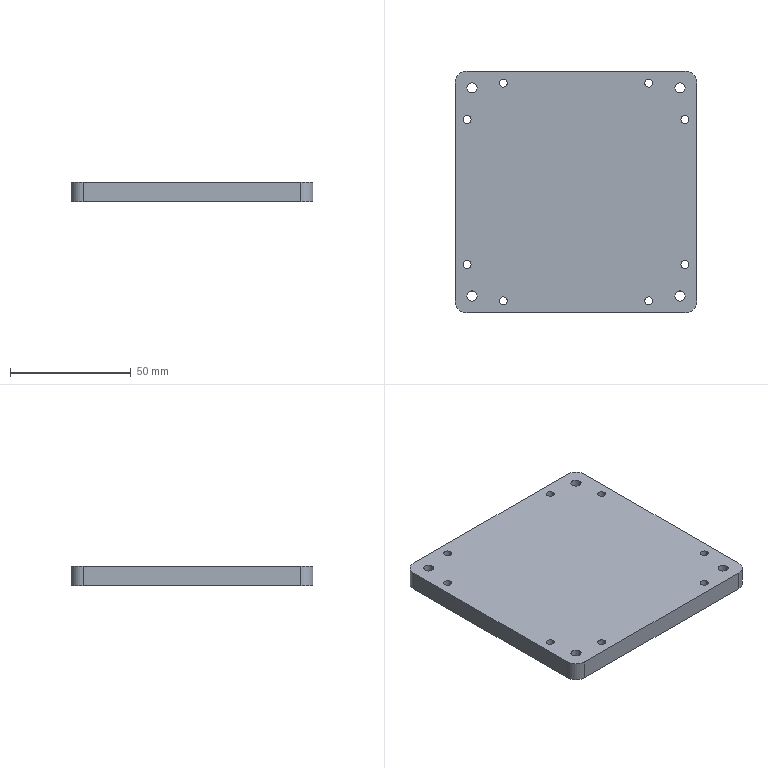Part | SolidWorks | features 3DProfileFeature 2, HoleWzd 2, Extrusion 1 | 1 solid | 34 faces | box 100 x 100 x 8 mm | volume 78838 mm3 | cylinder 28 | plane 6 | commonest cylinder face diameters 3.3 x16 4.2 x8 10 x4
STEP:
#1=CARTESIAN_POINT('',(-31.65,-45.,0.));
#2=VERTEX_POINT('',#1);
#3=CARTESIAN_POINT('',(-28.35,-45.,0.));
#4=VERTEX_POINT('',#3);
#5=CARTESIAN_POINT('',(-30.,-45.,0.));
#6=DIRECTION('',(0.,0.,1.));
#7=DIRECTION('',(1.,0.,0.));
#8=AXIS2_PLACEMENT_3D('',#5,#6,#7);
#9=CIRCLE('',#8,1.65);
#10=EDGE_CURVE('',#2,#4,#9,.T.);
#11=ORIENTED_EDGE('',*,*,#10,.F.);
#12=CARTESIAN_POINT('',(-31.65,-45.,8.));
#13=VERTEX_POINT('',#12);
#14=CARTESIAN_POINT('',(-31.65,-45.,8.));
#15=DIRECTION('',(0.,0.,1.));
#16=VECTOR('',#15,1000.);
#17=LINE('',#14,#16);
#18=EDGE_CURVE('',#2,#13,#17,.T.);
#19=ORIENTED_EDGE('',*,*,#18,.T.);
#20=CARTESIAN_POINT('',(-28.35,-45.,8.));
#21=VERTEX_POINT('',#20);
#22=CARTESIAN_POINT('',(-30.,-45.,8.));
#23=DIRECTION('',(0.,0.,1.));
#24=DIRECTION('',(1.,0.,0.));
#25=AXIS2_PLACEMENT_3D('',#22,#23,#24);
#26=CIRCLE('',#25,1.65);
#27=EDGE_CURVE('',#13,#21,#26,.T.);
#28=ORIENTED_EDGE('',*,*,#27,.T.);
#29=CARTESIAN_POINT('',(-28.35,-45.,8.));
#30=DIRECTION('',(0.,0.,1.));
#31=VECTOR('',#30,1000.);
#32=LINE('',#29,#31);
#33=EDGE_CURVE('',#4,#21,#32,.T.);
#34=ORIENTED_EDGE('',*,*,#33,.F.);
#35=EDGE_LOOP('',(#11,#19,#28,#34));
#36=FACE_OUTER_BOUND('',#35,.T.);
#37=CARTESIAN_POINT('',(-30.,-45.,8.));
#38=DIRECTION('',(0.,0.,1.));
#39=DIRECTION('',(1.,0.,0.));
#40=AXIS2_PLACEMENT_3D('',#37,#38,#39);
#41=CYLINDRICAL_SURFACE('',#40,1.65);
#42=ADVANCED_FACE('',(#36),#41,.F.);
#43=CARTESIAN_POINT('',(28.35,-45.,0.));
#44=VERTEX_POINT('',#43);
#45=CARTESIAN_POINT('',(31.65,-45.,0.));
#46=VERTEX_POINT('',#45);
#47=CARTESIAN_POINT('',(30.,-45.,0.));
#48=DIRECTION('',(0.,0.,1.));
#49=DIRECTION('',(1.,0.,0.));
#50=AXIS2_PLACEMENT_3D('',#47,#48,#49);
#51=CIRCLE('',#50,1.65);
#52=EDGE_CURVE('',#44,#46,#51,.T.);
#53=ORIENTED_EDGE('',*,*,#52,.F.);
#54=CARTESIAN_POINT('',(28.35,-45.,8.));
#55=VERTEX_POINT('',#54);
#56=CARTESIAN_POINT('',(28.35,-45.,8.));
#57=DIRECTION('',(0.,0.,1.));
#58=VECTOR('',#57,1000.);
#59=LINE('',#56,#58);
#60=EDGE_CURVE('',#44,#55,#59,.T.);
#61=ORIENTED_EDGE('',*,*,#60,.T.);
#62=CARTESIAN_POINT('',(31.65,-45.,8.));
#63=VERTEX_POINT('',#62);
#64=CARTESIAN_POINT('',(30.,-45.,8.));
#65=DIRECTION('',(0.,0.,1.));
#66=DIRECTION('',(1.,0.,0.));
#67=AXIS2_PLACEMENT_3D('',#64,#65,#66);
#68=CIRCLE('',#67,1.65);
#69=EDGE_CURVE('',#55,#63,#68,.T.);
#70=ORIENTED_EDGE('',*,*,#69,.T.);
#71=CARTESIAN_POINT('',(31.65,-45.,8.));
#72=DIRECTION('',(0.,0.,1.));
#73=VECTOR('',#72,1000.);
#74=LINE('',#71,#73);
#75=EDGE_CURVE('',#46,#63,#74,.T.);
#76=ORIENTED_EDGE('',*,*,#75,.F.);
#77=EDGE_LOOP('',(#53,#61,#70,#76));
#78=FACE_OUTER_BOUND('',#77,.T.);
#79=CARTESIAN_POINT('',(30.,-45.,8.));
#80=DIRECTION('',(0.,0.,1.));
#81=DIRECTION('',(1.,0.,0.));
#82=AXIS2_PLACEMENT_3D('',#79,#80,#81);
#83=CYLINDRICAL_SURFACE('',#82,1.65);
#84=ADVANCED_FACE('',(#78),#83,.F.);
#85=CARTESIAN_POINT('',(-46.65,-30.,0.));
#86=VERTEX_POINT('',#85);
#87=CARTESIAN_POINT('',(-43.35,-30.,0.));
#88=VERTEX_POINT('',#87);
#89=CARTESIAN_POINT('',(-45.,-30.,0.));
#90=DIRECTION('',(0.,0.,1.));
#91=DIRECTION('',(1.,0.,0.));
#92=AXIS2_PLACEMENT_3D('',#89,#90,#91);
#93=CIRCLE('',#92,1.65);
#94=EDGE_CURVE('',#86,#88,#93,.T.);
#95=ORIENTED_EDGE('',*,*,#94,.F.);
#96=CARTESIAN_POINT('',(-46.65,-30.,8.));
#97=VERTEX_POINT('',#96);
#98=CARTESIAN_POINT('',(-46.65,-30.,8.));
#99=DIRECTION('',(0.,0.,1.));
#100=VECTOR('',#99,1000.);
#101=LINE('',#98,#100);
#102=EDGE_CURVE('',#86,#97,#101,.T.);
#103=ORIENTED_EDGE('',*,*,#102,.T.);
#104=CARTESIAN_POINT('',(-43.35,-30.,8.));
#105=VERTEX_POINT('',#104);
#106=CARTESIAN_POINT('',(-45.,-30.,8.));
#107=DIRECTION('',(0.,0.,1.));
#108=DIRECTION('',(1.,0.,0.));
#109=AXIS2_PLACEMENT_3D('',#106,#107,#108);
#110=CIRCLE('',#109,1.65);
#111=EDGE_CURVE('',#97,#105,#110,.T.);
#112=ORIENTED_EDGE('',*,*,#111,.T.);
#113=CARTESIAN_POINT('',(-43.35,-30.,8.));
#114=DIRECTION('',(0.,0.,1.));
#115=VECTOR('',#114,1000.);
#116=LINE('',#113,#115);
#117=EDGE_CURVE('',#88,#105,#116,.T.);
#118=ORIENTED_EDGE('',*,*,#117,.F.);
#119=EDGE_LOOP('',(#95,#103,#112,#118));
#120=FACE_OUTER_BOUND('',#119,.T.);
#121=CARTESIAN_POINT('',(-45.,-30.,8.));
#122=DIRECTION('',(0.,0.,1.));
#123=DIRECTION('',(1.,0.,0.));
#124=AXIS2_PLACEMENT_3D('',#121,#122,#123);
#125=CYLINDRICAL_SURFACE('',#124,1.65);
#126=ADVANCED_FACE('',(#120),#125,.F.);
#127=CARTESIAN_POINT('',(-46.65,30.,0.));
#128=VERTEX_POINT('',#127);
#129=CARTESIAN_POINT('',(-43.35,30.,0.));
#130=VERTEX_POINT('',#129);
#131=CARTESIAN_POINT('',(-45.,30.,0.));
#132=DIRECTION('',(0.,0.,1.));
#133=DIRECTION('',(1.,0.,0.));
#134=AXIS2_PLACEMENT_3D('',#131,#132,#133);
#135=CIRCLE('',#134,1.65);
#136=EDGE_CURVE('',#128,#130,#135,.T.);
#137=ORIENTED_EDGE('',*,*,#136,.F.);
#138=CARTESIAN_POINT('',(-46.65,30.,8.));
#139=VERTEX_POINT('',#138);
#140=CARTESIAN_POINT('',(-46.65,30.,8.));
#141=DIRECTION('',(0.,0.,1.));
#142=VECTOR('',#141,1000.);
#143=LINE('',#140,#142);
#144=EDGE_CURVE('',#128,#139,#143,.T.);
#145=ORIENTED_EDGE('',*,*,#144,.T.);
#146=CARTESIAN_POINT('',(-43.35,30.,8.));
#147=VERTEX_POINT('',#146);
#148=CARTESIAN_POINT('',(-45.,30.,8.));
#149=DIRECTION('',(0.,0.,1.));
#150=DIRECTION('',(1.,0.,0.));
#151=AXIS2_PLACEMENT_3D('',#148,#149,#150);
#152=CIRCLE('',#151,1.65);
#153=EDGE_CURVE('',#139,#147,#152,.T.);
#154=ORIENTED_EDGE('',*,*,#153,.T.);
#155=CARTESIAN_POINT('',(-43.35,30.,8.));
#156=DIRECTION('',(0.,0.,1.));
#157=VECTOR('',#156,1000.);
#158=LINE('',#155,#157);
#159=EDGE_CURVE('',#130,#147,#158,.T.);
#160=ORIENTED_EDGE('',*,*,#159,.F.);
#161=EDGE_LOOP('',(#137,#145,#154,#160));
#162=FACE_OUTER_BOUND('',#161,.T.);
#163=CARTESIAN_POINT('',(-45.,30.,8.));
#164=DIRECTION('',(0.,0.,1.));
#165=DIRECTION('',(1.,0.,0.));
#166=AXIS2_PLACEMENT_3D('',#163,#164,#165);
#167=CYLINDRICAL_SURFACE('',#166,1.65);
#168=ADVANCED_FACE('',(#162),#167,.F.);
#169=CARTESIAN_POINT('',(43.35,30.,0.));
#170=VERTEX_POINT('',#169);
#171=CARTESIAN_POINT('',(46.65,30.,0.));
#172=VERTEX_POINT('',#171);
#173=CARTESIAN_POINT('',(45.,30.,0.));
#174=DIRECTION('',(0.,0.,1.));
#175=DIRECTION('',(1.,0.,0.));
#176=AXIS2_PLACEMENT_3D('',#173,#174,#175);
#177=CIRCLE('',#176,1.65);
#178=EDGE_CURVE('',#170,#172,#177,.T.);
#179=ORIENTED_EDGE('',*,*,#178,.F.);
#180=CARTESIAN_POINT('',(43.35,30.,8.));
#181=VERTEX_POINT('',#180);
#182=CARTESIAN_POINT('',(43.35,30.,8.));
#183=DIRECTION('',(0.,0.,1.));
#184=VECTOR('',#183,1000.);
#185=LINE('',#182,#184);
#186=EDGE_CURVE('',#170,#181,#185,.T.);
#187=ORIENTED_EDGE('',*,*,#186,.T.);
#188=CARTESIAN_POINT('',(46.65,30.,8.));
#189=VERTEX_POINT('',#188);
#190=CARTESIAN_POINT('',(45.,30.,8.));
#191=DIRECTION('',(0.,0.,1.));
#192=DIRECTION('',(1.,0.,0.));
#193=AXIS2_PLACEMENT_3D('',#190,#191,#192);
#194=CIRCLE('',#193,1.65);
#195=EDGE_CURVE('',#181,#189,#194,.T.);
#196=ORIENTED_EDGE('',*,*,#195,.T.);
#197=CARTESIAN_POINT('',(46.65,30.,8.));
#198=DIRECTION('',(0.,0.,1.));
#199=VECTOR('',#198,1000.);
#200=LINE('',#197,#199);
#201=EDGE_CURVE('',#172,#189,#200,.T.);
#202=ORIENTED_EDGE('',*,*,#201,.F.);
#203=EDGE_LOOP('',(#179,#187,#196,#202));
#204=FACE_OUTER_BOUND('',#203,.T.);
#205=CARTESIAN_POINT('',(45.,30.,8.));
#206=DIRECTION('',(0.,0.,1.));
#207=DIRECTION('',(1.,0.,0.));
#208=AXIS2_PLACEMENT_3D('',#205,#206,#207);
#209=CYLINDRICAL_SURFACE('',#208,1.65);
#210=ADVANCED_FACE('',(#204),#209,.F.);
#211=CARTESIAN_POINT('',(43.35,-30.,0.));
#212=VERTEX_POINT('',#211);
#213=CARTESIAN_POINT('',(46.65,-30.,0.));
#214=VERTEX_POINT('',#213);
#215=CARTESIAN_POINT('',(45.,-30.,0.));
#216=DIRECTION('',(0.,0.,1.));
#217=DIRECTION('',(1.,0.,0.));
#218=AXIS2_PLACEMENT_3D('',#215,#216,#217);
#219=CIRCLE('',#218,1.65);
#220=EDGE_CURVE('',#212,#214,#219,.T.);
#221=ORIENTED_EDGE('',*,*,#220,.F.);
#222=CARTESIAN_POINT('',(43.35,-30.,8.));
#223=VERTEX_POINT('',#222);
#224=CARTESIAN_POINT('',(43.35,-30.,8.));
#225=DIRECTION('',(0.,0.,1.));
#226=VECTOR('',#225,1000.);
#227=LINE('',#224,#226);
#228=EDGE_CURVE('',#212,#223,#227,.T.);
#229=ORIENTED_EDGE('',*,*,#228,.T.);
#230=CARTESIAN_POINT('',(46.65,-30.,8.));
#231=VERTEX_POINT('',#230);
#232=CARTESIAN_POINT('',(45.,-30.,8.));
#233=DIRECTION('',(0.,0.,1.));
#234=DIRECTION('',(1.,0.,0.));
#235=AXIS2_PLACEMENT_3D('',#232,#233,#234);
#236=CIRCLE('',#235,1.65);
#237=EDGE_CURVE('',#223,#231,#236,.T.);
#238=ORIENTED_EDGE('',*,*,#237,.T.);
#239=CARTESIAN_POINT('',(46.65,-30.,8.));
#240=DIRECTION('',(0.,0.,1.));
#241=VECTOR('',#240,1000.);
#242=LINE('',#239,#241);
#243=EDGE_CURVE('',#214,#231,#242,.T.);
#244=ORIENTED_EDGE('',*,*,#243,.F.);
#245=EDGE_LOOP('',(#221,#229,#238,#244));
#246=FACE_OUTER_BOUND('',#245,.T.);
#247=CARTESIAN_POINT('',(45.,-30.,8.));
#248=DIRECTION('',(0.,0.,1.));
#249=DIRECTION('',(1.,0.,0.));
#250=AXIS2_PLACEMENT_3D('',#247,#248,#249);
#251=CYLINDRICAL_SURFACE('',#250,1.65);
#252=ADVANCED_FACE('',(#246),#251,.F.);
#253=CARTESIAN_POINT('',(-31.65,45.,0.));
#254=VERTEX_POINT('',#253);
#255=CARTESIAN_POINT('',(-28.35,45.,0.));
#256=VERTEX_POINT('',#255);
#257=CARTESIAN_POINT('',(-30.,45.,0.));
#258=DIRECTION('',(0.,0.,1.));
#259=DIRECTION('',(1.,0.,0.));
#260=AXIS2_PLACEMENT_3D('',#257,#258,#259);
#261=CIRCLE('',#260,1.65);
#262=EDGE_CURVE('',#254,#256,#261,.T.);
#263=ORIENTED_EDGE('',*,*,#262,.F.);
#264=CARTESIAN_POINT('',(-31.65,45.,8.));
#265=VERTEX_POINT('',#264);
#266=CARTESIAN_POINT('',(-31.65,45.,8.));
#267=DIRECTION('',(0.,0.,1.));
#268=VECTOR('',#267,1000.);
#269=LINE('',#266,#268);
#270=EDGE_CURVE('',#254,#265,#269,.T.);
#271=ORIENTED_EDGE('',*,*,#270,.T.);
#272=CARTESIAN_POINT('',(-28.35,45.,8.));
#273=VERTEX_POINT('',#272);
#274=CARTESIAN_POINT('',(-30.,45.,8.));
#275=DIRECTION('',(0.,0.,1.));
#276=DIRECTION('',(1.,0.,0.));
#277=AXIS2_PLACEMENT_3D('',#274,#275,#276);
#278=CIRCLE('',#277,1.65);
#279=EDGE_CURVE('',#265,#273,#278,.T.);
#280=ORIENTED_EDGE('',*,*,#279,.T.);
#281=CARTESIAN_POINT('',(-28.35,45.,8.));
#282=DIRECTION('',(0.,0.,1.));
#283=VECTOR('',#282,1000.);
#284=LINE('',#281,#283);
#285=EDGE_CURVE('',#256,#273,#284,.T.);
#286=ORIENTED_EDGE('',*,*,#285,.F.);
#287=EDGE_LOOP('',(#263,#271,#280,#286));
#288=FACE_OUTER_BOUND('',#287,.T.);
#289=CARTESIAN_POINT('',(-30.,45.,8.));
#290=DIRECTION('',(0.,0.,1.));
#291=DIRECTION('',(1.,0.,0.));
#292=AXIS2_PLACEMENT_3D('',#289,#290,#291);
#293=CYLINDRICAL_SURFACE('',#292,1.65);
#294=ADVANCED_FACE('',(#288),#293,.F.);
#295=CARTESIAN_POINT('',(28.35,45.,0.));
#296=VERTEX_POINT('',#295);
#297=CARTESIAN_POINT('',(31.65,45.,0.));
#298=VERTEX_POINT('',#297);
#299=CARTESIAN_POINT('',(30.,45.,0.));
#300=DIRECTION('',(0.,0.,1.));
#301=DIRECTION('',(1.,0.,0.));
#302=AXIS2_PLACEMENT_3D('',#299,#300,#301);
#303=CIRCLE('',#302,1.65);
#304=EDGE_CURVE('',#296,#298,#303,.T.);
#305=ORIENTED_EDGE('',*,*,#304,.F.);
#306=CARTESIAN_POINT('',(28.35,45.,8.));
#307=VERTEX_POINT('',#306);
#308=CARTESIAN_POINT('',(28.35,45.,8.));
#309=DIRECTION('',(0.,0.,1.));
#310=VECTOR('',#309,1000.);
#311=LINE('',#308,#310);
#312=EDGE_CURVE('',#296,#307,#311,.T.);
#313=ORIENTED_EDGE('',*,*,#312,.T.);
#314=CARTESIAN_POINT('',(31.65,45.,8.));
#315=VERTEX_POINT('',#314);
#316=CARTESIAN_POINT('',(30.,45.,8.));
#317=DIRECTION('',(0.,0.,1.));
#318=DIRECTION('',(1.,0.,0.));
#319=AXIS2_PLACEMENT_3D('',#316,#317,#318);
#320=CIRCLE('',#319,1.65);
#321=EDGE_CURVE('',#307,#315,#320,.T.);
#322=ORIENTED_EDGE('',*,*,#321,.T.);
#323=CARTESIAN_POINT('',(31.65,45.,8.));
#324=DIRECTION('',(0.,0.,1.));
#325=VECTOR('',#324,1000.);
#326=LINE('',#323,#325);
#327=EDGE_CURVE('',#298,#315,#326,.T.);
#328=ORIENTED_EDGE('',*,*,#327,.F.);
#329=EDGE_LOOP('',(#305,#313,#322,#328));
#330=FACE_OUTER_BOUND('',#329,.T.);
#331=CARTESIAN_POINT('',(30.,45.,8.));
#332=DIRECTION('',(0.,0.,1.));
#333=DIRECTION('',(1.,0.,0.));
#334=AXIS2_PLACEMENT_3D('',#331,#332,#333);
#335=CYLINDRICAL_SURFACE('',#334,1.65);
#336=ADVANCED_FACE('',(#330),#335,.F.);
#337=CARTESIAN_POINT('',(-45.1,43.,0.));
#338=VERTEX_POINT('',#337);
#339=CARTESIAN_POINT('',(-40.9,43.,0.));
#340=VERTEX_POINT('',#339);
#341=CARTESIAN_POINT('',(-43.,43.,0.));
#342=DIRECTION('',(0.,0.,1.));
#343=DIRECTION('',(1.,0.,0.));
#344=AXIS2_PLACEMENT_3D('',#341,#342,#343);
#345=CIRCLE('',#344,2.1);
#346=EDGE_CURVE('',#338,#340,#345,.T.);
#347=ORIENTED_EDGE('',*,*,#346,.F.);
#348=CARTESIAN_POINT('',(-45.1,43.,8.));
#349=VERTEX_POINT('',#348);
#350=CARTESIAN_POINT('',(-45.1,43.,8.));
#351=DIRECTION('',(0.,0.,1.));
#352=VECTOR('',#351,1000.);
#353=LINE('',#350,#352);
#354=EDGE_CURVE('',#338,#349,#353,.T.);
#355=ORIENTED_EDGE('',*,*,#354,.T.);
#356=CARTESIAN_POINT('',(-40.9,43.,8.));
#357=VERTEX_POINT('',#356);
#358=CARTESIAN_POINT('',(-43.,43.,8.));
#359=DIRECTION('',(0.,0.,1.));
#360=DIRECTION('',(1.,0.,0.));
#361=AXIS2_PLACEMENT_3D('',#358,#359,#360);
#362=CIRCLE('',#361,2.1);
#363=EDGE_CURVE('',#349,#357,#362,.T.);
#364=ORIENTED_EDGE('',*,*,#363,.T.);
#365=CARTESIAN_POINT('',(-40.9,43.,8.));
#366=DIRECTION('',(0.,0.,1.));
#367=VECTOR('',#366,1000.);
#368=LINE('',#365,#367);
#369=EDGE_CURVE('',#340,#357,#368,.T.);
#370=ORIENTED_EDGE('',*,*,#369,.F.);
#371=EDGE_LOOP('',(#347,#355,#364,#370));
#372=FACE_OUTER_BOUND('',#371,.T.);
#373=CARTESIAN_POINT('',(-43.,43.,8.));
#374=DIRECTION('',(0.,0.,1.));
#375=DIRECTION('',(1.,0.,0.));
#376=AXIS2_PLACEMENT_3D('',#373,#374,#375);
#377=CYLINDRICAL_SURFACE('',#376,2.1);
#378=ADVANCED_FACE('',(#372),#377,.F.);
#379=CARTESIAN_POINT('',(40.9,43.,0.));
#380=VERTEX_POINT('',#379);
#381=CARTESIAN_POINT('',(45.1,43.,0.));
#382=VERTEX_POINT('',#381);
#383=CARTESIAN_POINT('',(43.,43.,0.));
#384=DIRECTION('',(0.,0.,1.));
#385=DIRECTION('',(1.,0.,0.));
#386=AXIS2_PLACEMENT_3D('',#383,#384,#385);
#387=CIRCLE('',#386,2.1);
#388=EDGE_CURVE('',#380,#382,#387,.T.);
#389=ORIENTED_EDGE('',*,*,#388,.F.);
#390=CARTESIAN_POINT('',(40.9,43.,8.));
#391=VERTEX_POINT('',#390);
#392=CARTESIAN_POINT('',(40.9,43.,8.));
#393=DIRECTION('',(0.,0.,1.));
#394=VECTOR('',#393,1000.);
#395=LINE('',#392,#394);
#396=EDGE_CURVE('',#380,#391,#395,.T.);
#397=ORIENTED_EDGE('',*,*,#396,.T.);
#398=CARTESIAN_POINT('',(45.1,43.,8.));
#399=VERTEX_POINT('',#398);
#400=CARTESIAN_POINT('',(43.,43.,8.));
#401=DIRECTION('',(0.,0.,1.));
#402=DIRECTION('',(1.,0.,0.));
#403=AXIS2_PLACEMENT_3D('',#400,#401,#402);
#404=CIRCLE('',#403,2.1);
#405=EDGE_CURVE('',#391,#399,#404,.T.);
#406=ORIENTED_EDGE('',*,*,#405,.T.);
#407=CARTESIAN_POINT('',(45.1,43.,8.));
#408=DIRECTION('',(0.,0.,1.));
#409=VECTOR('',#408,1000.);
#410=LINE('',#407,#409);
#411=EDGE_CURVE('',#382,#399,#410,.T.);
#412=ORIENTED_EDGE('',*,*,#411,.F.);
#413=EDGE_LOOP('',(#389,#397,#406,#412));
#414=FACE_OUTER_BOUND('',#413,.T.);
#415=CARTESIAN_POINT('',(43.,43.,8.));
#416=DIRECTION('',(0.,0.,1.));
#417=DIRECTION('',(1.,0.,0.));
#418=AXIS2_PLACEMENT_3D('',#415,#416,#417);
#419=CYLINDRICAL_SURFACE('',#418,2.1);
#420=ADVANCED_FACE('',(#414),#419,.F.);
#421=CARTESIAN_POINT('',(40.9,-43.,0.));
#422=VERTEX_POINT('',#421);
#423=CARTESIAN_POINT('',(45.1,-43.,0.));
#424=VERTEX_POINT('',#423);
#425=CARTESIAN_POINT('',(43.,-43.,0.));
#426=DIRECTION('',(0.,0.,1.));
#427=DIRECTION('',(1.,0.,0.));
#428=AXIS2_PLACEMENT_3D('',#425,#426,#427);
#429=CIRCLE('',#428,2.1);
#430=EDGE_CURVE('',#422,#424,#429,.T.);
#431=ORIENTED_EDGE('',*,*,#430,.F.);
#432=CARTESIAN_POINT('',(40.9,-43.,8.));
#433=VERTEX_POINT('',#432);
#434=CARTESIAN_POINT('',(40.9,-43.,8.));
#435=DIRECTION('',(0.,0.,1.));
#436=VECTOR('',#435,1000.);
#437=LINE('',#434,#436);
#438=EDGE_CURVE('',#422,#433,#437,.T.);
#439=ORIENTED_EDGE('',*,*,#438,.T.);
#440=CARTESIAN_POINT('',(45.1,-43.,8.));
#441=VERTEX_POINT('',#440);
#442=CARTESIAN_POINT('',(43.,-43.,8.));
#443=DIRECTION('',(0.,0.,1.));
#444=DIRECTION('',(1.,0.,0.));
#445=AXIS2_PLACEMENT_3D('',#442,#443,#444);
#446=CIRCLE('',#445,2.1);
#447=EDGE_CURVE('',#433,#441,#446,.T.);
#448=ORIENTED_EDGE('',*,*,#447,.T.);
#449=CARTESIAN_POINT('',(45.1,-43.,8.));
#450=DIRECTION('',(0.,0.,1.));
#451=VECTOR('',#450,1000.);
#452=LINE('',#449,#451);
#453=EDGE_CURVE('',#424,#441,#452,.T.);
#454=ORIENTED_EDGE('',*,*,#453,.F.);
#455=EDGE_LOOP('',(#431,#439,#448,#454));
#456=FACE_OUTER_BOUND('',#455,.T.);
#457=CARTESIAN_POINT('',(43.,-43.,8.));
#458=DIRECTION('',(0.,0.,1.));
#459=DIRECTION('',(1.,0.,0.));
#460=AXIS2_PLACEMENT_3D('',#457,#458,#459);
#461=CYLINDRICAL_SURFACE('',#460,2.1);
#462=ADVANCED_FACE('',(#456),#461,.F.);
#463=CARTESIAN_POINT('',(-45.1,-43.,0.));
#464=VERTEX_POINT('',#463);
#465=CARTESIAN_POINT('',(-40.9,-43.,0.));
#466=VERTEX_POINT('',#465);
#467=CARTESIAN_POINT('',(-43.,-43.,0.));
#468=DIRECTION('',(0.,0.,1.));
#469=DIRECTION('',(1.,0.,0.));
#470=AXIS2_PLACEMENT_3D('',#467,#468,#469);
#471=CIRCLE('',#470,2.1);
#472=EDGE_CURVE('',#464,#466,#471,.T.);
#473=ORIENTED_EDGE('',*,*,#472,.F.);
#474=CARTESIAN_POINT('',(-45.1,-43.,8.));
#475=VERTEX_POINT('',#474);
#476=CARTESIAN_POINT('',(-45.1,-43.,8.));
#477=DIRECTION('',(0.,0.,1.));
#478=VECTOR('',#477,1000.);
#479=LINE('',#476,#478);
#480=EDGE_CURVE('',#464,#475,#479,.T.);
#481=ORIENTED_EDGE('',*,*,#480,.T.);
#482=CARTESIAN_POINT('',(-40.9,-43.,8.));
#483=VERTEX_POINT('',#482);
#484=CARTESIAN_POINT('',(-43.,-43.,8.));
#485=DIRECTION('',(0.,0.,1.));
#486=DIRECTION('',(1.,0.,0.));
#487=AXIS2_PLACEMENT_3D('',#484,#485,#486);
#488=CIRCLE('',#487,2.1);
#489=EDGE_CURVE('',#475,#483,#488,.T.);
#490=ORIENTED_EDGE('',*,*,#489,.T.);
#491=CARTESIAN_POINT('',(-40.9,-43.,8.));
#492=DIRECTION('',(0.,0.,1.));
#493=VECTOR('',#492,1000.);
#494=LINE('',#491,#493);
#495=EDGE_CURVE('',#466,#483,#494,.T.);
#496=ORIENTED_EDGE('',*,*,#495,.F.);
#497=EDGE_LOOP('',(#473,#481,#490,#496));
#498=FACE_OUTER_BOUND('',#497,.T.);
#499=CARTESIAN_POINT('',(-43.,-43.,8.));
#500=DIRECTION('',(0.,0.,1.));
#501=DIRECTION('',(1.,0.,0.));
#502=AXIS2_PLACEMENT_3D('',#499,#500,#501);
#503=CYLINDRICAL_SURFACE('',#502,2.1);
#504=ADVANCED_FACE('',(#498),#503,.F.);
#505=CARTESIAN_POINT('',(45.,-50.,0.));
#506=VERTEX_POINT('',#505);
#507=CARTESIAN_POINT('',(50.,-45.,0.));
#508=VERTEX_POINT('',#507);
#509=CARTESIAN_POINT('',(45.,-45.,0.));
#510=DIRECTION('',(0.,0.,1.));
#511=DIRECTION('',(1.,0.,0.));
#512=AXIS2_PLACEMENT_3D('',#509,#510,#511);
#513=CIRCLE('',#512,5.);
#514=EDGE_CURVE('',#506,#508,#513,.T.);
#515=ORIENTED_EDGE('',*,*,#514,.T.);
#516=CARTESIAN_POINT('',(50.,-45.,8.));
#517=VERTEX_POINT('',#516);
#518=CARTESIAN_POINT('',(50.,-45.,8.));
#519=DIRECTION('',(0.,0.,-1.));
#520=VECTOR('',#519,1000.);
#521=LINE('',#518,#520);
#522=EDGE_CURVE('',#517,#508,#521,.T.);
#523=ORIENTED_EDGE('',*,*,#522,.F.);
#524=CARTESIAN_POINT('',(45.,-50.,8.));
#525=VERTEX_POINT('',#524);
#526=CARTESIAN_POINT('',(45.,-45.,8.));
#527=DIRECTION('',(0.,0.,1.));
#528=DIRECTION('',(1.,0.,0.));
#529=AXIS2_PLACEMENT_3D('',#526,#527,#528);
#530=CIRCLE('',#529,5.);
#531=EDGE_CURVE('',#525,#517,#530,.T.);
#532=ORIENTED_EDGE('',*,*,#531,.F.);
#533=CARTESIAN_POINT('',(45.,-50.,8.));
#534=DIRECTION('',(0.,0.,-1.));
#535=VECTOR('',#534,1000.);
#536=LINE('',#533,#535);
#537=EDGE_CURVE('',#525,#506,#536,.T.);
#538=ORIENTED_EDGE('',*,*,#537,.T.);
#539=EDGE_LOOP('',(#515,#523,#532,#538));
#540=FACE_OUTER_BOUND('',#539,.T.);
#541=CARTESIAN_POINT('',(45.,-45.,8.));
#542=DIRECTION('',(0.,0.,-1.));
#543=DIRECTION('',(-1.,0.,0.));
#544=AXIS2_PLACEMENT_3D('',#541,#542,#543);
#545=CYLINDRICAL_SURFACE('',#544,5.);
#546=ADVANCED_FACE('',(#540),#545,.T.);
#547=CARTESIAN_POINT('',(50.,45.,0.));
#548=VERTEX_POINT('',#547);
#549=CARTESIAN_POINT('',(50.,45.,0.));
#550=DIRECTION('',(0.,1.,0.));
#551=VECTOR('',#550,1000.);
#552=LINE('',#549,#551);
#553=EDGE_CURVE('',#508,#548,#552,.T.);
#554=ORIENTED_EDGE('',*,*,#553,.T.);
#555=CARTESIAN_POINT('',(50.,45.,8.));
#556=VERTEX_POINT('',#555);
#557=CARTESIAN_POINT('',(50.,45.,8.));
#558=DIRECTION('',(0.,0.,-1.));
#559=VECTOR('',#558,1000.);
#560=LINE('',#557,#559);
#561=EDGE_CURVE('',#556,#548,#560,.T.);
#562=ORIENTED_EDGE('',*,*,#561,.F.);
#563=CARTESIAN_POINT('',(50.,45.,8.));
#564=DIRECTION('',(0.,1.,0.));
#565=VECTOR('',#564,1000.);
#566=LINE('',#563,#565);
#567=EDGE_CURVE('',#517,#556,#566,.T.);
#568=ORIENTED_EDGE('',*,*,#567,.F.);
#569=ORIENTED_EDGE('',*,*,#522,.T.);
#570=EDGE_LOOP('',(#554,#562,#568,#569));
#571=FACE_OUTER_BOUND('',#570,.T.);
#572=CARTESIAN_POINT('',(50.,45.,8.));
#573=DIRECTION('',(-1.,0.,0.));
#574=DIRECTION('',(0.,-1.,0.));
#575=AXIS2_PLACEMENT_3D('',#572,#573,#574);
#576=PLANE('',#575);
#577=ADVANCED_FACE('',(#571),#576,.F.);
#578=CARTESIAN_POINT('',(45.,50.,0.));
#579=VERTEX_POINT('',#578);
#580=CARTESIAN_POINT('',(45.,45.,0.));
#581=DIRECTION('',(0.,0.,1.));
#582=DIRECTION('',(-1.,0.,0.));
#583=AXIS2_PLACEMENT_3D('',#580,#581,#582);
#584=CIRCLE('',#583,5.);
#585=EDGE_CURVE('',#548,#579,#584,.T.);
#586=ORIENTED_EDGE('',*,*,#585,.T.);
#587=CARTESIAN_POINT('',(45.,50.,8.));
#588=VERTEX_POINT('',#587);
#589=CARTESIAN_POINT('',(45.,50.,8.));
#590=DIRECTION('',(0.,0.,-1.));
#591=VECTOR('',#590,1000.);
#592=LINE('',#589,#591);
#593=EDGE_CURVE('',#588,#579,#592,.T.);
#594=ORIENTED_EDGE('',*,*,#593,.F.);
#595=CARTESIAN_POINT('',(45.,45.,8.));
#596=DIRECTION('',(0.,0.,1.));
#597=DIRECTION('',(-1.,0.,0.));
#598=AXIS2_PLACEMENT_3D('',#595,#596,#597);
#599=CIRCLE('',#598,5.);
#600=EDGE_CURVE('',#556,#588,#599,.T.);
#601=ORIENTED_EDGE('',*,*,#600,.F.);
#602=ORIENTED_EDGE('',*,*,#561,.T.);
#603=EDGE_LOOP('',(#586,#594,#601,#602));
#604=FACE_OUTER_BOUND('',#603,.T.);
#605=CARTESIAN_POINT('',(45.,45.,8.));
#606=DIRECTION('',(0.,0.,-1.));
#607=DIRECTION('',(-1.,0.,0.));
#608=AXIS2_PLACEMENT_3D('',#605,#606,#607);
#609=CYLINDRICAL_SURFACE('',#608,5.);
#610=ADVANCED_FACE('',(#604),#609,.T.);
#611=CARTESIAN_POINT('',(-45.,50.,0.));
#612=VERTEX_POINT('',#611);
#613=CARTESIAN_POINT('',(-45.,50.,0.));
#614=DIRECTION('',(-1.,0.,0.));
#615=VECTOR('',#614,1000.);
#616=LINE('',#613,#615);
#617=EDGE_CURVE('',#579,#612,#616,.T.);
#618=ORIENTED_EDGE('',*,*,#617,.T.);
#619=CARTESIAN_POINT('',(-45.,50.,8.));
#620=VERTEX_POINT('',#619);
#621=CARTESIAN_POINT('',(-45.,50.,8.));
#622=DIRECTION('',(0.,0.,-1.));
#623=VECTOR('',#622,1000.);
#624=LINE('',#621,#623);
#625=EDGE_CURVE('',#620,#612,#624,.T.);
#626=ORIENTED_EDGE('',*,*,#625,.F.);
#627=CARTESIAN_POINT('',(-45.,50.,8.));
#628=DIRECTION('',(-1.,0.,0.));
#629=VECTOR('',#628,1000.);
#630=LINE('',#627,#629);
#631=EDGE_CURVE('',#588,#620,#630,.T.);
#632=ORIENTED_EDGE('',*,*,#631,.F.);
#633=ORIENTED_EDGE('',*,*,#593,.T.);
#634=EDGE_LOOP('',(#618,#626,#632,#633));
#635=FACE_OUTER_BOUND('',#634,.T.);
#636=CARTESIAN_POINT('',(-45.,50.,8.));
#637=DIRECTION('',(0.,-1.,0.));
#638=DIRECTION('',(0.,0.,-1.));
#639=AXIS2_PLACEMENT_3D('',#636,#637,#638);
#640=PLANE('',#639);
#641=ADVANCED_FACE('',(#635),#640,.F.);
#642=CARTESIAN_POINT('',(-50.,45.,0.));
#643=VERTEX_POINT('',#642);
#644=CARTESIAN_POINT('',(-45.,45.,0.));
#645=DIRECTION('',(0.,0.,1.));
#646=DIRECTION('',(1.,0.,0.));
#647=AXIS2_PLACEMENT_3D('',#644,#645,#646);
#648=CIRCLE('',#647,5.);
#649=EDGE_CURVE('',#612,#643,#648,.T.);
#650=ORIENTED_EDGE('',*,*,#649,.T.);
#651=CARTESIAN_POINT('',(-50.,45.,8.));
#652=VERTEX_POINT('',#651);
#653=CARTESIAN_POINT('',(-50.,45.,8.));
#654=DIRECTION('',(0.,0.,-1.));
#655=VECTOR('',#654,1000.);
#656=LINE('',#653,#655);
#657=EDGE_CURVE('',#652,#643,#656,.T.);
#658=ORIENTED_EDGE('',*,*,#657,.F.);
#659=CARTESIAN_POINT('',(-45.,45.,8.));
#660=DIRECTION('',(0.,0.,1.));
#661=DIRECTION('',(1.,0.,0.));
#662=AXIS2_PLACEMENT_3D('',#659,#660,#661);
#663=CIRCLE('',#662,5.);
#664=EDGE_CURVE('',#620,#652,#663,.T.);
#665=ORIENTED_EDGE('',*,*,#664,.F.);
#666=ORIENTED_EDGE('',*,*,#625,.T.);
#667=EDGE_LOOP('',(#650,#658,#665,#666));
#668=FACE_OUTER_BOUND('',#667,.T.);
#669=CARTESIAN_POINT('',(-45.,45.,8.));
#670=DIRECTION('',(0.,0.,-1.));
#671=DIRECTION('',(-1.,0.,0.));
#672=AXIS2_PLACEMENT_3D('',#669,#670,#671);
#673=CYLINDRICAL_SURFACE('',#672,5.);
#674=ADVANCED_FACE('',(#668),#673,.T.);
#675=CARTESIAN_POINT('',(-50.,-45.,0.));
#676=VERTEX_POINT('',#675);
#677=CARTESIAN_POINT('',(-50.,45.,0.));
#678=DIRECTION('',(0.,-1.,0.));
#679=VECTOR('',#678,1000.);
#680=LINE('',#677,#679);
#681=EDGE_CURVE('',#643,#676,#680,.T.);
#682=ORIENTED_EDGE('',*,*,#681,.T.);
#683=CARTESIAN_POINT('',(-50.,-45.,8.));
#684=VERTEX_POINT('',#683);
#685=CARTESIAN_POINT('',(-50.,-45.,8.));
#686=DIRECTION('',(0.,0.,-1.));
#687=VECTOR('',#686,1000.);
#688=LINE('',#685,#687);
#689=EDGE_CURVE('',#684,#676,#688,.T.);
#690=ORIENTED_EDGE('',*,*,#689,.F.);
#691=CARTESIAN_POINT('',(-50.,45.,8.));
#692=DIRECTION('',(0.,-1.,0.));
#693=VECTOR('',#692,1000.);
#694=LINE('',#691,#693);
#695=EDGE_CURVE('',#652,#684,#694,.T.);
#696=ORIENTED_EDGE('',*,*,#695,.F.);
#697=ORIENTED_EDGE('',*,*,#657,.T.);
#698=EDGE_LOOP('',(#682,#690,#696,#697));
#699=FACE_OUTER_BOUND('',#698,.T.);
#700=CARTESIAN_POINT('',(-50.,45.,8.));
#701=DIRECTION('',(1.,0.,0.));
#702=DIRECTION('',(0.,1.,0.));
#703=AXIS2_PLACEMENT_3D('',#700,#701,#702);
#704=PLANE('',#703);
#705=ADVANCED_FACE('',(#699),#704,.F.);
#706=CARTESIAN_POINT('',(-45.,-50.,0.));
#707=VERTEX_POINT('',#706);
#708=CARTESIAN_POINT('',(-45.,-45.,0.));
#709=DIRECTION('',(0.,0.,1.));
#710=DIRECTION('',(1.,0.,0.));
#711=AXIS2_PLACEMENT_3D('',#708,#709,#710);
#712=CIRCLE('',#711,5.);
#713=EDGE_CURVE('',#676,#707,#712,.T.);
#714=ORIENTED_EDGE('',*,*,#713,.T.);
#715=CARTESIAN_POINT('',(-45.,-50.,8.));
#716=VERTEX_POINT('',#715);
#717=CARTESIAN_POINT('',(-45.,-50.,8.));
#718=DIRECTION('',(0.,0.,-1.));
#719=VECTOR('',#718,1000.);
#720=LINE('',#717,#719);
#721=EDGE_CURVE('',#716,#707,#720,.T.);
#722=ORIENTED_EDGE('',*,*,#721,.F.);
#723=CARTESIAN_POINT('',(-45.,-45.,8.));
#724=DIRECTION('',(0.,0.,1.));
#725=DIRECTION('',(1.,0.,0.));
#726=AXIS2_PLACEMENT_3D('',#723,#724,#725);
#727=CIRCLE('',#726,5.);
#728=EDGE_CURVE('',#684,#716,#727,.T.);
#729=ORIENTED_EDGE('',*,*,#728,.F.);
#730=ORIENTED_EDGE('',*,*,#689,.T.);
#731=EDGE_LOOP('',(#714,#722,#729,#730));
#732=FACE_OUTER_BOUND('',#731,.T.);
#733=CARTESIAN_POINT('',(-45.,-45.,8.));
#734=DIRECTION('',(0.,0.,-1.));
#735=DIRECTION('',(-1.,0.,0.));
#736=AXIS2_PLACEMENT_3D('',#733,#734,#735);
#737=CYLINDRICAL_SURFACE('',#736,5.);
#738=ADVANCED_FACE('',(#732),#737,.T.);
#739=CARTESIAN_POINT('',(-45.,-50.,0.));
#740=DIRECTION('',(1.,0.,0.));
#741=VECTOR('',#740,1000.);
#742=LINE('',#739,#741);
#743=EDGE_CURVE('',#707,#506,#742,.T.);
#744=ORIENTED_EDGE('',*,*,#743,.T.);
#745=ORIENTED_EDGE('',*,*,#537,.F.);
#746=CARTESIAN_POINT('',(-45.,-50.,8.));
#747=DIRECTION('',(1.,0.,0.));
#748=VECTOR('',#747,1000.);
#749=LINE('',#746,#748);
#750=EDGE_CURVE('',#716,#525,#749,.T.);
#751=ORIENTED_EDGE('',*,*,#750,.F.);
#752=ORIENTED_EDGE('',*,*,#721,.T.);
#753=EDGE_LOOP('',(#744,#745,#751,#752));
#754=FACE_OUTER_BOUND('',#753,.T.);
#755=CARTESIAN_POINT('',(-45.,-50.,8.));
#756=DIRECTION('',(0.,1.,0.));
#757=DIRECTION('',(0.,0.,1.));
#758=AXIS2_PLACEMENT_3D('',#755,#756,#757);
#759=PLANE('',#758);
#760=ADVANCED_FACE('',(#754),#759,.F.);
#761=CARTESIAN_POINT('',(-30.,-45.,8.));
#762=DIRECTION('',(0.,0.,1.));
#763=DIRECTION('',(1.,0.,0.));
#764=AXIS2_PLACEMENT_3D('',#761,#762,#763);
#765=CIRCLE('',#764,1.65);
#766=EDGE_CURVE('',#21,#13,#765,.T.);
#767=ORIENTED_EDGE('',*,*,#766,.F.);
#768=ORIENTED_EDGE('',*,*,#27,.F.);
#769=EDGE_LOOP('',(#767,#768));
#770=FACE_BOUND('',#769,.T.);
#771=CARTESIAN_POINT('',(30.,-45.,8.));
#772=DIRECTION('',(0.,0.,1.));
#773=DIRECTION('',(1.,0.,0.));
#774=AXIS2_PLACEMENT_3D('',#771,#772,#773);
#775=CIRCLE('',#774,1.65);
#776=EDGE_CURVE('',#63,#55,#775,.T.);
#777=ORIENTED_EDGE('',*,*,#776,.F.);
#778=ORIENTED_EDGE('',*,*,#69,.F.);
#779=EDGE_LOOP('',(#777,#778));
#780=FACE_BOUND('',#779,.T.);
#781=CARTESIAN_POINT('',(-45.,-30.,8.));
#782=DIRECTION('',(0.,0.,1.));
#783=DIRECTION('',(1.,0.,0.));
#784=AXIS2_PLACEMENT_3D('',#781,#782,#783);
#785=CIRCLE('',#784,1.65);
#786=EDGE_CURVE('',#105,#97,#785,.T.);
#787=ORIENTED_EDGE('',*,*,#786,.F.);
#788=ORIENTED_EDGE('',*,*,#111,.F.);
#789=EDGE_LOOP('',(#787,#788));
#790=FACE_BOUND('',#789,.T.);
#791=CARTESIAN_POINT('',(-45.,30.,8.));
#792=DIRECTION('',(0.,0.,1.));
#793=DIRECTION('',(1.,0.,0.));
#794=AXIS2_PLACEMENT_3D('',#791,#792,#793);
#795=CIRCLE('',#794,1.65);
#796=EDGE_CURVE('',#147,#139,#795,.T.);
#797=ORIENTED_EDGE('',*,*,#796,.F.);
#798=ORIENTED_EDGE('',*,*,#153,.F.);
#799=EDGE_LOOP('',(#797,#798));
#800=FACE_BOUND('',#799,.T.);
#801=CARTESIAN_POINT('',(45.,30.,8.));
#802=DIRECTION('',(0.,0.,1.));
#803=DIRECTION('',(1.,0.,0.));
#804=AXIS2_PLACEMENT_3D('',#801,#802,#803);
#805=CIRCLE('',#804,1.65);
#806=EDGE_CURVE('',#189,#181,#805,.T.);
#807=ORIENTED_EDGE('',*,*,#806,.F.);
#808=ORIENTED_EDGE('',*,*,#195,.F.);
#809=EDGE_LOOP('',(#807,#808));
#810=FACE_BOUND('',#809,.T.);
#811=CARTESIAN_POINT('',(45.,-30.,8.));
#812=DIRECTION('',(0.,0.,1.));
#813=DIRECTION('',(1.,0.,0.));
#814=AXIS2_PLACEMENT_3D('',#811,#812,#813);
#815=CIRCLE('',#814,1.65);
#816=EDGE_CURVE('',#231,#223,#815,.T.);
#817=ORIENTED_EDGE('',*,*,#816,.F.);
#818=ORIENTED_EDGE('',*,*,#237,.F.);
#819=EDGE_LOOP('',(#817,#818));
#820=FACE_BOUND('',#819,.T.);
#821=CARTESIAN_POINT('',(-30.,45.,8.));
#822=DIRECTION('',(0.,0.,1.));
#823=DIRECTION('',(1.,0.,0.));
#824=AXIS2_PLACEMENT_3D('',#821,#822,#823);
#825=CIRCLE('',#824,1.65);
#826=EDGE_CURVE('',#273,#265,#825,.T.);
#827=ORIENTED_EDGE('',*,*,#826,.F.);
#828=ORIENTED_EDGE('',*,*,#279,.F.);
#829=EDGE_LOOP('',(#827,#828));
#830=FACE_BOUND('',#829,.T.);
#831=CARTESIAN_POINT('',(30.,45.,8.));
#832=DIRECTION('',(0.,0.,1.));
#833=DIRECTION('',(1.,0.,0.));
#834=AXIS2_PLACEMENT_3D('',#831,#832,#833);
#835=CIRCLE('',#834,1.65);
#836=EDGE_CURVE('',#315,#307,#835,.T.);
#837=ORIENTED_EDGE('',*,*,#836,.F.);
#838=ORIENTED_EDGE('',*,*,#321,.F.);
#839=EDGE_LOOP('',(#837,#838));
#840=FACE_BOUND('',#839,.T.);
#841=CARTESIAN_POINT('',(-43.,43.,8.));
#842=DIRECTION('',(0.,0.,1.));
#843=DIRECTION('',(1.,0.,0.));
#844=AXIS2_PLACEMENT_3D('',#841,#842,#843);
#845=CIRCLE('',#844,2.1);
#846=EDGE_CURVE('',#357,#349,#845,.T.);
#847=ORIENTED_EDGE('',*,*,#846,.F.);
#848=ORIENTED_EDGE('',*,*,#363,.F.);
#849=EDGE_LOOP('',(#847,#848));
#850=FACE_BOUND('',#849,.T.);
#851=CARTESIAN_POINT('',(43.,43.,8.));
#852=DIRECTION('',(0.,0.,1.));
#853=DIRECTION('',(1.,0.,0.));
#854=AXIS2_PLACEMENT_3D('',#851,#852,#853);
#855=CIRCLE('',#854,2.1);
#856=EDGE_CURVE('',#399,#391,#855,.T.);
#857=ORIENTED_EDGE('',*,*,#856,.F.);
#858=ORIENTED_EDGE('',*,*,#405,.F.);
#859=EDGE_LOOP('',(#857,#858));
#860=FACE_BOUND('',#859,.T.);
#861=CARTESIAN_POINT('',(43.,-43.,8.));
#862=DIRECTION('',(0.,0.,1.));
#863=DIRECTION('',(1.,0.,0.));
#864=AXIS2_PLACEMENT_3D('',#861,#862,#863);
#865=CIRCLE('',#864,2.1);
#866=EDGE_CURVE('',#441,#433,#865,.T.);
#867=ORIENTED_EDGE('',*,*,#866,.F.);
#868=ORIENTED_EDGE('',*,*,#447,.F.);
#869=EDGE_LOOP('',(#867,#868));
#870=FACE_BOUND('',#869,.T.);
#871=CARTESIAN_POINT('',(-43.,-43.,8.));
#872=DIRECTION('',(0.,0.,1.));
#873=DIRECTION('',(1.,0.,0.));
#874=AXIS2_PLACEMENT_3D('',#871,#872,#873);
#875=CIRCLE('',#874,2.1);
#876=EDGE_CURVE('',#483,#475,#875,.T.);
#877=ORIENTED_EDGE('',*,*,#876,.F.);
#878=ORIENTED_EDGE('',*,*,#489,.F.);
#879=EDGE_LOOP('',(#877,#878));
#880=FACE_BOUND('',#879,.T.);
#881=ORIENTED_EDGE('',*,*,#531,.T.);
#882=ORIENTED_EDGE('',*,*,#567,.T.);
#883=ORIENTED_EDGE('',*,*,#600,.T.);
#884=ORIENTED_EDGE('',*,*,#631,.T.);
#885=ORIENTED_EDGE('',*,*,#664,.T.);
#886=ORIENTED_EDGE('',*,*,#695,.T.);
#887=ORIENTED_EDGE('',*,*,#728,.T.);
#888=ORIENTED_EDGE('',*,*,#750,.T.);
#889=EDGE_LOOP('',(#881,#882,#883,#884,#885,#886,#887,#888));
#890=FACE_OUTER_BOUND('',#889,.T.);
#891=CARTESIAN_POINT('',(45.,-45.,8.));
#892=DIRECTION('',(0.,0.,1.));
#893=DIRECTION('',(1.,0.,0.));
#894=AXIS2_PLACEMENT_3D('',#891,#892,#893);
#895=PLANE('',#894);
#896=ADVANCED_FACE('',(#770,#780,#790,#800,#810,#820,#830,#840,#850,#860,#870,#880,#890),#895,.T.);
#897=CARTESIAN_POINT('',(-30.,-45.,0.));
#898=DIRECTION('',(0.,0.,1.));
#899=DIRECTION('',(1.,0.,0.));
#900=AXIS2_PLACEMENT_3D('',#897,#898,#899);
#901=CIRCLE('',#900,1.65);
#902=EDGE_CURVE('',#4,#2,#901,.T.);
#903=ORIENTED_EDGE('',*,*,#902,.T.);
#904=ORIENTED_EDGE('',*,*,#10,.T.);
#905=EDGE_LOOP('',(#903,#904));
#906=FACE_BOUND('',#905,.T.);
#907=CARTESIAN_POINT('',(30.,-45.,0.));
#908=DIRECTION('',(0.,0.,1.));
#909=DIRECTION('',(1.,0.,0.));
#910=AXIS2_PLACEMENT_3D('',#907,#908,#909);
#911=CIRCLE('',#910,1.65);
#912=EDGE_CURVE('',#46,#44,#911,.T.);
#913=ORIENTED_EDGE('',*,*,#912,.T.);
#914=ORIENTED_EDGE('',*,*,#52,.T.);
#915=EDGE_LOOP('',(#913,#914));
#916=FACE_BOUND('',#915,.T.);
#917=CARTESIAN_POINT('',(-45.,-30.,0.));
#918=DIRECTION('',(0.,0.,1.));
#919=DIRECTION('',(1.,0.,0.));
#920=AXIS2_PLACEMENT_3D('',#917,#918,#919);
#921=CIRCLE('',#920,1.65);
#922=EDGE_CURVE('',#88,#86,#921,.T.);
#923=ORIENTED_EDGE('',*,*,#922,.T.);
#924=ORIENTED_EDGE('',*,*,#94,.T.);
#925=EDGE_LOOP('',(#923,#924));
#926=FACE_BOUND('',#925,.T.);
#927=CARTESIAN_POINT('',(-45.,30.,0.));
#928=DIRECTION('',(0.,0.,1.));
#929=DIRECTION('',(1.,0.,0.));
#930=AXIS2_PLACEMENT_3D('',#927,#928,#929);
#931=CIRCLE('',#930,1.65);
#932=EDGE_CURVE('',#130,#128,#931,.T.);
#933=ORIENTED_EDGE('',*,*,#932,.T.);
#934=ORIENTED_EDGE('',*,*,#136,.T.);
#935=EDGE_LOOP('',(#933,#934));
#936=FACE_BOUND('',#935,.T.);
#937=CARTESIAN_POINT('',(45.,30.,0.));
#938=DIRECTION('',(0.,0.,1.));
#939=DIRECTION('',(1.,0.,0.));
#940=AXIS2_PLACEMENT_3D('',#937,#938,#939);
#941=CIRCLE('',#940,1.65);
#942=EDGE_CURVE('',#172,#170,#941,.T.);
#943=ORIENTED_EDGE('',*,*,#942,.T.);
#944=ORIENTED_EDGE('',*,*,#178,.T.);
#945=EDGE_LOOP('',(#943,#944));
#946=FACE_BOUND('',#945,.T.);
#947=CARTESIAN_POINT('',(45.,-30.,0.));
#948=DIRECTION('',(0.,0.,1.));
#949=DIRECTION('',(1.,0.,0.));
#950=AXIS2_PLACEMENT_3D('',#947,#948,#949);
#951=CIRCLE('',#950,1.65);
#952=EDGE_CURVE('',#214,#212,#951,.T.);
#953=ORIENTED_EDGE('',*,*,#952,.T.);
#954=ORIENTED_EDGE('',*,*,#220,.T.);
#955=EDGE_LOOP('',(#953,#954));
#956=FACE_BOUND('',#955,.T.);
#957=CARTESIAN_POINT('',(-30.,45.,0.));
#958=DIRECTION('',(0.,0.,1.));
#959=DIRECTION('',(1.,0.,0.));
#960=AXIS2_PLACEMENT_3D('',#957,#958,#959);
#961=CIRCLE('',#960,1.65);
#962=EDGE_CURVE('',#256,#254,#961,.T.);
#963=ORIENTED_EDGE('',*,*,#962,.T.);
#964=ORIENTED_EDGE('',*,*,#262,.T.);
#965=EDGE_LOOP('',(#963,#964));
#966=FACE_BOUND('',#965,.T.);
#967=CARTESIAN_POINT('',(30.,45.,0.));
#968=DIRECTION('',(0.,0.,1.));
#969=DIRECTION('',(1.,0.,0.));
#970=AXIS2_PLACEMENT_3D('',#967,#968,#969);
#971=CIRCLE('',#970,1.65);
#972=EDGE_CURVE('',#298,#296,#971,.T.);
#973=ORIENTED_EDGE('',*,*,#972,.T.);
#974=ORIENTED_EDGE('',*,*,#304,.T.);
#975=EDGE_LOOP('',(#973,#974));
#976=FACE_BOUND('',#975,.T.);
#977=CARTESIAN_POINT('',(-43.,43.,0.));
#978=DIRECTION('',(0.,0.,1.));
#979=DIRECTION('',(1.,0.,0.));
#980=AXIS2_PLACEMENT_3D('',#977,#978,#979);
#981=CIRCLE('',#980,2.1);
#982=EDGE_CURVE('',#340,#338,#981,.T.);
#983=ORIENTED_EDGE('',*,*,#982,.T.);
#984=ORIENTED_EDGE('',*,*,#346,.T.);
#985=EDGE_LOOP('',(#983,#984));
#986=FACE_BOUND('',#985,.T.);
#987=CARTESIAN_POINT('',(43.,43.,0.));
#988=DIRECTION('',(0.,0.,1.));
#989=DIRECTION('',(1.,0.,0.));
#990=AXIS2_PLACEMENT_3D('',#987,#988,#989);
#991=CIRCLE('',#990,2.1);
#992=EDGE_CURVE('',#382,#380,#991,.T.);
#993=ORIENTED_EDGE('',*,*,#992,.T.);
#994=ORIENTED_EDGE('',*,*,#388,.T.);
#995=EDGE_LOOP('',(#993,#994));
#996=FACE_BOUND('',#995,.T.);
#997=CARTESIAN_POINT('',(43.,-43.,0.));
#998=DIRECTION('',(0.,0.,1.));
#999=DIRECTION('',(1.,0.,0.));
#1000=AXIS2_PLACEMENT_3D('',#997,#998,#999);
#1001=CIRCLE('',#1000,2.1);
#1002=EDGE_CURVE('',#424,#422,#1001,.T.);
#1003=ORIENTED_EDGE('',*,*,#1002,.T.);
#1004=ORIENTED_EDGE('',*,*,#430,.T.);
#1005=EDGE_LOOP('',(#1003,#1004));
#1006=FACE_BOUND('',#1005,.T.);
#1007=CARTESIAN_POINT('',(-43.,-43.,0.));
#1008=DIRECTION('',(0.,0.,1.));
#1009=DIRECTION('',(1.,0.,0.));
#1010=AXIS2_PLACEMENT_3D('',#1007,#1008,#1009);
#1011=CIRCLE('',#1010,2.1);
#1012=EDGE_CURVE('',#466,#464,#1011,.T.);
#1013=ORIENTED_EDGE('',*,*,#1012,.T.);
#1014=ORIENTED_EDGE('',*,*,#472,.T.);
#1015=EDGE_LOOP('',(#1013,#1014));
#1016=FACE_BOUND('',#1015,.T.);
#1017=ORIENTED_EDGE('',*,*,#514,.F.);
#1018=ORIENTED_EDGE('',*,*,#743,.F.);
#1019=ORIENTED_EDGE('',*,*,#713,.F.);
#1020=ORIENTED_EDGE('',*,*,#681,.F.);
#1021=ORIENTED_EDGE('',*,*,#649,.F.);
#1022=ORIENTED_EDGE('',*,*,#617,.F.);
#1023=ORIENTED_EDGE('',*,*,#585,.F.);
#1024=ORIENTED_EDGE('',*,*,#553,.F.);
#1025=EDGE_LOOP('',(#1017,#1018,#1019,#1020,#1021,#1022,#1023,#1024));
#1026=FACE_OUTER_BOUND('',#1025,.T.);
#1027=CARTESIAN_POINT('',(45.,-45.,0.));
#1028=DIRECTION('',(0.,0.,1.));
#1029=DIRECTION('',(1.,0.,0.));
#1030=AXIS2_PLACEMENT_3D('',#1027,#1028,#1029);
#1031=PLANE('',#1030);
#1032=ADVANCED_FACE('',(#906,#916,#926,#936,#946,#956,#966,#976,#986,#996,#1006,#1016,#1026),#1031,.F.);
#1033=ORIENTED_EDGE('',*,*,#480,.F.);
#1034=ORIENTED_EDGE('',*,*,#1012,.F.);
#1035=ORIENTED_EDGE('',*,*,#495,.T.);
#1036=ORIENTED_EDGE('',*,*,#876,.T.);
#1037=EDGE_LOOP('',(#1033,#1034,#1035,#1036));
#1038=FACE_OUTER_BOUND('',#1037,.T.);
#1039=CARTESIAN_POINT('',(-43.,-43.,8.));
#1040=DIRECTION('',(0.,0.,1.));
#1041=DIRECTION('',(1.,0.,0.));
#1042=AXIS2_PLACEMENT_3D('',#1039,#1040,#1041);
#1043=CYLINDRICAL_SURFACE('',#1042,2.1);
#1044=ADVANCED_FACE('',(#1038),#1043,.F.);
#1045=ORIENTED_EDGE('',*,*,#438,.F.);
#1046=ORIENTED_EDGE('',*,*,#1002,.F.);
#1047=ORIENTED_EDGE('',*,*,#453,.T.);
#1048=ORIENTED_EDGE('',*,*,#866,.T.);
#1049=EDGE_LOOP('',(#1045,#1046,#1047,#1048));
#1050=FACE_OUTER_BOUND('',#1049,.T.);
#1051=CARTESIAN_POINT('',(43.,-43.,8.));
#1052=DIRECTION('',(0.,0.,1.));
#1053=DIRECTION('',(1.,0.,0.));
#1054=AXIS2_PLACEMENT_3D('',#1051,#1052,#1053);
#1055=CYLINDRICAL_SURFACE('',#1054,2.1);
#1056=ADVANCED_FACE('',(#1050),#1055,.F.);
#1057=ORIENTED_EDGE('',*,*,#396,.F.);
#1058=ORIENTED_EDGE('',*,*,#992,.F.);
#1059=ORIENTED_EDGE('',*,*,#411,.T.);
#1060=ORIENTED_EDGE('',*,*,#856,.T.);
#1061=EDGE_LOOP('',(#1057,#1058,#1059,#1060));
#1062=FACE_OUTER_BOUND('',#1061,.T.);
#1063=CARTESIAN_POINT('',(43.,43.,8.));
#1064=DIRECTION('',(0.,0.,1.));
#1065=DIRECTION('',(1.,0.,0.));
#1066=AXIS2_PLACEMENT_3D('',#1063,#1064,#1065);
#1067=CYLINDRICAL_SURFACE('',#1066,2.1);
#1068=ADVANCED_FACE('',(#1062),#1067,.F.);
#1069=ORIENTED_EDGE('',*,*,#354,.F.);
#1070=ORIENTED_EDGE('',*,*,#982,.F.);
#1071=ORIENTED_EDGE('',*,*,#369,.T.);
#1072=ORIENTED_EDGE('',*,*,#846,.T.);
#1073=EDGE_LOOP('',(#1069,#1070,#1071,#1072));
#1074=FACE_OUTER_BOUND('',#1073,.T.);
#1075=CARTESIAN_POINT('',(-43.,43.,8.));
#1076=DIRECTION('',(0.,0.,1.));
#1077=DIRECTION('',(1.,0.,0.));
#1078=AXIS2_PLACEMENT_3D('',#1075,#1076,#1077);
#1079=CYLINDRICAL_SURFACE('',#1078,2.1);
#1080=ADVANCED_FACE('',(#1074),#1079,.F.);
#1081=ORIENTED_EDGE('',*,*,#312,.F.);
#1082=ORIENTED_EDGE('',*,*,#972,.F.);
#1083=ORIENTED_EDGE('',*,*,#327,.T.);
#1084=ORIENTED_EDGE('',*,*,#836,.T.);
#1085=EDGE_LOOP('',(#1081,#1082,#1083,#1084));
#1086=FACE_OUTER_BOUND('',#1085,.T.);
#1087=CARTESIAN_POINT('',(30.,45.,8.));
#1088=DIRECTION('',(0.,0.,1.));
#1089=DIRECTION('',(1.,0.,0.));
#1090=AXIS2_PLACEMENT_3D('',#1087,#1088,#1089);
#1091=CYLINDRICAL_SURFACE('',#1090,1.65);
#1092=ADVANCED_FACE('',(#1086),#1091,.F.);
#1093=ORIENTED_EDGE('',*,*,#270,.F.);
#1094=ORIENTED_EDGE('',*,*,#962,.F.);
#1095=ORIENTED_EDGE('',*,*,#285,.T.);
#1096=ORIENTED_EDGE('',*,*,#826,.T.);
#1097=EDGE_LOOP('',(#1093,#1094,#1095,#1096));
#1098=FACE_OUTER_BOUND('',#1097,.T.);
#1099=CARTESIAN_POINT('',(-30.,45.,8.));
#1100=DIRECTION('',(0.,0.,1.));
#1101=DIRECTION('',(1.,0.,0.));
#1102=AXIS2_PLACEMENT_3D('',#1099,#1100,#1101);
#1103=CYLINDRICAL_SURFACE('',#1102,1.65);
#1104=ADVANCED_FACE('',(#1098),#1103,.F.);
#1105=ORIENTED_EDGE('',*,*,#228,.F.);
#1106=ORIENTED_EDGE('',*,*,#952,.F.);
#1107=ORIENTED_EDGE('',*,*,#243,.T.);
#1108=ORIENTED_EDGE('',*,*,#816,.T.);
#1109=EDGE_LOOP('',(#1105,#1106,#1107,#1108));
#1110=FACE_OUTER_BOUND('',#1109,.T.);
#1111=CARTESIAN_POINT('',(45.,-30.,8.));
#1112=DIRECTION('',(0.,0.,1.));
#1113=DIRECTION('',(1.,0.,0.));
#1114=AXIS2_PLACEMENT_3D('',#1111,#1112,#1113);
#1115=CYLINDRICAL_SURFACE('',#1114,1.65);
#1116=ADVANCED_FACE('',(#1110),#1115,.F.);
#1117=ORIENTED_EDGE('',*,*,#186,.F.);
#1118=ORIENTED_EDGE('',*,*,#942,.F.);
#1119=ORIENTED_EDGE('',*,*,#201,.T.);
#1120=ORIENTED_EDGE('',*,*,#806,.T.);
#1121=EDGE_LOOP('',(#1117,#1118,#1119,#1120));
#1122=FACE_OUTER_BOUND('',#1121,.T.);
#1123=CARTESIAN_POINT('',(45.,30.,8.));
#1124=DIRECTION('',(0.,0.,1.));
#1125=DIRECTION('',(1.,0.,0.));
#1126=AXIS2_PLACEMENT_3D('',#1123,#1124,#1125);
#1127=CYLINDRICAL_SURFACE('',#1126,1.65);
#1128=ADVANCED_FACE('',(#1122),#1127,.F.);
#1129=ORIENTED_EDGE('',*,*,#144,.F.);
#1130=ORIENTED_EDGE('',*,*,#932,.F.);
#1131=ORIENTED_EDGE('',*,*,#159,.T.);
#1132=ORIENTED_EDGE('',*,*,#796,.T.);
#1133=EDGE_LOOP('',(#1129,#1130,#1131,#1132));
#1134=FACE_OUTER_BOUND('',#1133,.T.);
#1135=CARTESIAN_POINT('',(-45.,30.,8.));
#1136=DIRECTION('',(0.,0.,1.));
#1137=DIRECTION('',(1.,0.,0.));
#1138=AXIS2_PLACEMENT_3D('',#1135,#1136,#1137);
#1139=CYLINDRICAL_SURFACE('',#1138,1.65);
#1140=ADVANCED_FACE('',(#1134),#1139,.F.);
#1141=ORIENTED_EDGE('',*,*,#102,.F.);
#1142=ORIENTED_EDGE('',*,*,#922,.F.);
#1143=ORIENTED_EDGE('',*,*,#117,.T.);
#1144=ORIENTED_EDGE('',*,*,#786,.T.);
#1145=EDGE_LOOP('',(#1141,#1142,#1143,#1144));
#1146=FACE_OUTER_BOUND('',#1145,.T.);
#1147=CARTESIAN_POINT('',(-45.,-30.,8.));
#1148=DIRECTION('',(0.,0.,1.));
#1149=DIRECTION('',(1.,0.,0.));
#1150=AXIS2_PLACEMENT_3D('',#1147,#1148,#1149);
#1151=CYLINDRICAL_SURFACE('',#1150,1.65);
#1152=ADVANCED_FACE('',(#1146),#1151,.F.);
#1153=ORIENTED_EDGE('',*,*,#60,.F.);
#1154=ORIENTED_EDGE('',*,*,#912,.F.);
#1155=ORIENTED_EDGE('',*,*,#75,.T.);
#1156=ORIENTED_EDGE('',*,*,#776,.T.);
#1157=EDGE_LOOP('',(#1153,#1154,#1155,#1156));
#1158=FACE_OUTER_BOUND('',#1157,.T.);
#1159=CARTESIAN_POINT('',(30.,-45.,8.));
#1160=DIRECTION('',(0.,0.,1.));
#1161=DIRECTION('',(1.,0.,0.));
#1162=AXIS2_PLACEMENT_3D('',#1159,#1160,#1161);
#1163=CYLINDRICAL_SURFACE('',#1162,1.65);
#1164=ADVANCED_FACE('',(#1158),#1163,.F.);
#1165=ORIENTED_EDGE('',*,*,#18,.F.);
#1166=ORIENTED_EDGE('',*,*,#902,.F.);
#1167=ORIENTED_EDGE('',*,*,#33,.T.);
#1168=ORIENTED_EDGE('',*,*,#766,.T.);
#1169=EDGE_LOOP('',(#1165,#1166,#1167,#1168));
#1170=FACE_OUTER_BOUND('',#1169,.T.);
#1171=CARTESIAN_POINT('',(-30.,-45.,8.));
#1172=DIRECTION('',(0.,0.,1.));
#1173=DIRECTION('',(1.,0.,0.));
#1174=AXIS2_PLACEMENT_3D('',#1171,#1172,#1173);
#1175=CYLINDRICAL_SURFACE('',#1174,1.65);
#1176=ADVANCED_FACE('',(#1170),#1175,.F.);
#1177=CLOSED_SHELL('',(#42,#84,#126,#168,#210,#252,#294,#336,#378,#420,#462,#504,#546,#577,#610,#641,#674,#705,#738,#760,#896,#1032,#1044,#1056,#1068,#1080,#1092,#1104,#1116,#1128,#1140,#1152,#1164,#1176));
#1178=MANIFOLD_SOLID_BREP('',#1177);
#1179=CARTESIAN_POINT('',(0.,0.,0.));
#1180=DIRECTION('',(0.,0.,1.));
#1181=DIRECTION('',(1.,0.,0.));
#1182=AXIS2_PLACEMENT_3D('',#1179,#1180,#1181);
#1183=(LENGTH_UNIT()NAMED_UNIT(*)SI_UNIT(.MILLI.,.METRE.));
#1184=UNCERTAINTY_MEASURE_WITH_UNIT(LENGTH_MEASURE(0.00001),#1183,'','');
#1185=(NAMED_UNIT(*)PLANE_ANGLE_UNIT()SI_UNIT($,.RADIAN.));
#1186=(NAMED_UNIT(*)SI_UNIT($,.STERADIAN.)SOLID_ANGLE_UNIT());
#1187=(GEOMETRIC_REPRESENTATION_CONTEXT(3)GLOBAL_UNCERTAINTY_ASSIGNED_CONTEXT((#1184))GLOBAL_UNIT_ASSIGNED_CONTEXT((#1183,#1185,#1186))REPRESENTATION_CONTEXT('',''));
#1188=ADVANCED_BREP_SHAPE_REPRESENTATION('',(#1178,#1182),#1187);